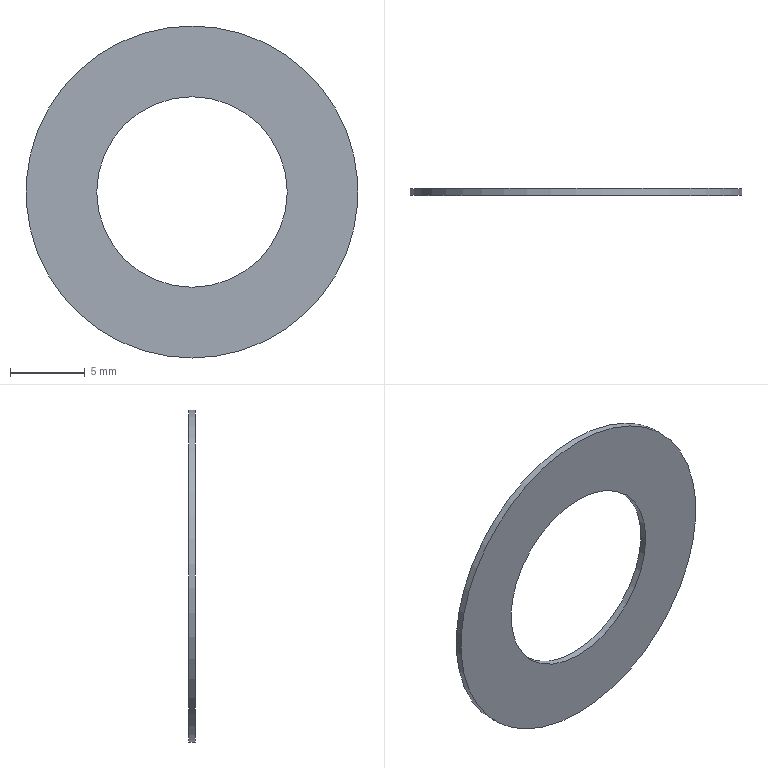Part | NX | features piston flapper 2 | 1 solid | 4 faces | box 22.225 x 0.4572 x 22.225 mm | volume 118.989 mm3 | cylinder 2 | plane 2 | commonest cylinder face diameters 12.751 x1 22.225 x1
STEP:
#1=CARTESIAN_POINT('',(0.,31.21,-6.375));
#2=VERTEX_POINT('',#1);
#3=CARTESIAN_POINT('',(0.,31.21,0.));
#4=DIRECTION('',(0.,-1.,0.));
#5=DIRECTION('',(0.,0.,-1.));
#6=AXIS2_PLACEMENT_3D('',#3,#4,#5);
#7=CIRCLE('',#6,6.375);
#8=EDGE_CURVE('',#2,#2,#7,.T.);
#9=ORIENTED_EDGE('',*,*,#8,.T.);
#10=EDGE_LOOP('',(#9));
#11=FACE_BOUND('',#10,.T.);
#12=CARTESIAN_POINT('',(0.,31.667,-6.375));
#13=VERTEX_POINT('',#12);
#14=CARTESIAN_POINT('',(0.,31.667,0.));
#15=DIRECTION('',(0.,-1.,0.));
#16=DIRECTION('',(0.,0.,-1.));
#17=AXIS2_PLACEMENT_3D('',#14,#15,#16);
#18=CIRCLE('',#17,6.375);
#19=EDGE_CURVE('',#13,#13,#18,.T.);
#20=ORIENTED_EDGE('',*,*,#19,.F.);
#21=EDGE_LOOP('',(#20));
#22=FACE_BOUND('',#21,.T.);
#23=CARTESIAN_POINT('',(0.,0.,0.));
#24=DIRECTION('',(0.,-1.,0.));
#25=DIRECTION('',(0.,0.,-1.));
#26=AXIS2_PLACEMENT_3D('',#23,#24,#25);
#27=CYLINDRICAL_SURFACE('',#26,6.375);
#28=ADVANCED_FACE('',(#11,#22),#27,.F.);
#29=CARTESIAN_POINT('',(0.,31.21,-11.113));
#30=VERTEX_POINT('',#29);
#31=CARTESIAN_POINT('',(0.,31.21,0.));
#32=DIRECTION('',(0.,-1.,0.));
#33=DIRECTION('',(0.,0.,-1.));
#34=AXIS2_PLACEMENT_3D('',#31,#32,#33);
#35=CIRCLE('',#34,11.113);
#36=EDGE_CURVE('',#30,#30,#35,.T.);
#37=ORIENTED_EDGE('',*,*,#36,.T.);
#38=EDGE_LOOP('',(#37));
#39=FACE_BOUND('',#38,.T.);
#40=ORIENTED_EDGE('',*,*,#8,.F.);
#41=EDGE_LOOP('',(#40));
#42=FACE_BOUND('',#41,.T.);
#43=CARTESIAN_POINT('',(6.375,31.21,0.));
#44=DIRECTION('',(0.,-1.,0.));
#45=DIRECTION('',(0.,0.,-1.));
#46=AXIS2_PLACEMENT_3D('',#43,#44,#45);
#47=PLANE('',#46);
#48=ADVANCED_FACE('',(#39,#42),#47,.T.);
#49=CARTESIAN_POINT('',(0.,31.667,-11.113));
#50=VERTEX_POINT('',#49);
#51=CARTESIAN_POINT('',(0.,31.667,0.));
#52=DIRECTION('',(0.,-1.,0.));
#53=DIRECTION('',(0.,0.,-1.));
#54=AXIS2_PLACEMENT_3D('',#51,#52,#53);
#55=CIRCLE('',#54,11.113);
#56=EDGE_CURVE('',#50,#50,#55,.T.);
#57=ORIENTED_EDGE('',*,*,#56,.T.);
#58=EDGE_LOOP('',(#57));
#59=FACE_BOUND('',#58,.T.);
#60=ORIENTED_EDGE('',*,*,#36,.F.);
#61=EDGE_LOOP('',(#60));
#62=FACE_BOUND('',#61,.T.);
#63=CARTESIAN_POINT('',(0.,0.,0.));
#64=DIRECTION('',(0.,-1.,0.));
#65=DIRECTION('',(0.,0.,-1.));
#66=AXIS2_PLACEMENT_3D('',#63,#64,#65);
#67=CYLINDRICAL_SURFACE('',#66,11.113);
#68=ADVANCED_FACE('',(#59,#62),#67,.T.);
#69=ORIENTED_EDGE('',*,*,#19,.T.);
#70=EDGE_LOOP('',(#69));
#71=FACE_BOUND('',#70,.T.);
#72=ORIENTED_EDGE('',*,*,#56,.F.);
#73=EDGE_LOOP('',(#72));
#74=FACE_BOUND('',#73,.T.);
#75=CARTESIAN_POINT('',(6.375,31.667,0.));
#76=DIRECTION('',(0.,1.,0.));
#77=DIRECTION('',(0.,0.,1.));
#78=AXIS2_PLACEMENT_3D('',#75,#76,#77);
#79=PLANE('',#78);
#80=ADVANCED_FACE('',(#71,#74),#79,.T.);
#81=CLOSED_SHELL('',(#28,#48,#68,#80));
#82=MANIFOLD_SOLID_BREP('',#81);
#83=(LENGTH_UNIT()NAMED_UNIT(*)SI_UNIT(.MILLI.,.METRE.));
#84=UNCERTAINTY_MEASURE_WITH_UNIT(LENGTH_MEASURE(0.00001),#83,'','');
#85=(NAMED_UNIT(*)PLANE_ANGLE_UNIT()SI_UNIT($,.RADIAN.));
#86=(NAMED_UNIT(*)SI_UNIT($,.STERADIAN.)SOLID_ANGLE_UNIT());
#87=(GEOMETRIC_REPRESENTATION_CONTEXT(3)GLOBAL_UNCERTAINTY_ASSIGNED_CONTEXT((#84))GLOBAL_UNIT_ASSIGNED_CONTEXT((#83,#85,#86))REPRESENTATION_CONTEXT('',''));
#88=ADVANCED_BREP_SHAPE_REPRESENTATION('',(#82),#87);